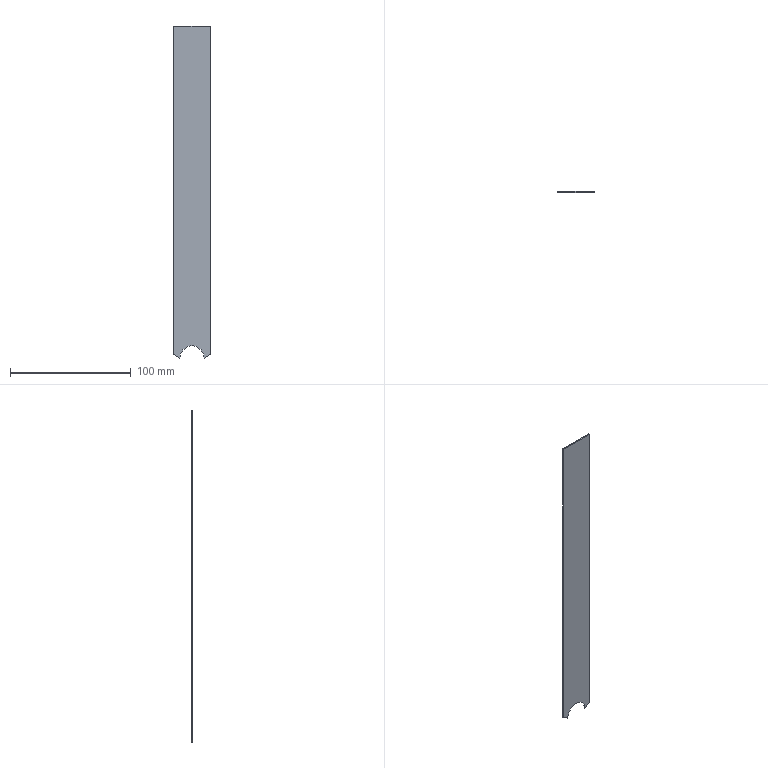Part | STEP file | solid 160 | 1 solid | 10 faces | box 30.5 x 1 x 274.425 mm | volume 8203 mm3 | plane 5 | cylinder 3 | cone 2 | commonest cylinder face diameters 30.5 x2 20 x1